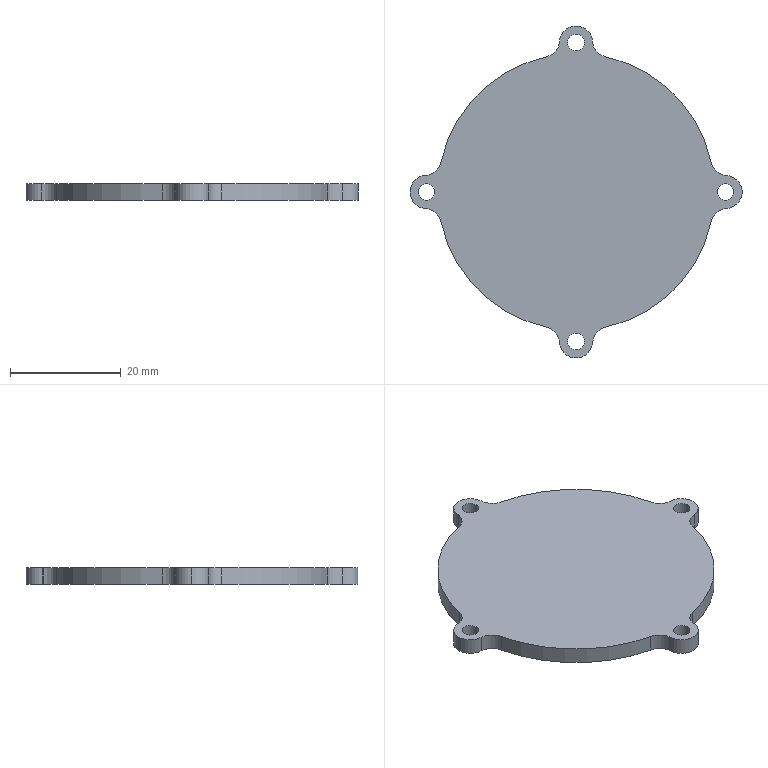Part | SolidWorks | features Extrusion 1 | 1 solid | 31 faces | box 60 x 60 x 3 mm | volume 6153 mm3 | cylinder 29 | plane 2 | commonest cylinder face diameters 6 x15 3 x8 50 x4 54 x2
STEP:
#1=CARTESIAN_POINT('',(-28.5,0.,3.));
#2=VERTEX_POINT('',#1);
#3=CARTESIAN_POINT('',(-25.5,0.,3.));
#4=VERTEX_POINT('',#3);
#5=CARTESIAN_POINT('',(-27.,0.,3.));
#6=DIRECTION('',(0.,0.,1.));
#7=DIRECTION('',(1.,0.,0.));
#8=AXIS2_PLACEMENT_3D('',#5,#6,#7);
#9=CIRCLE('',#8,1.5);
#10=EDGE_CURVE('',#2,#4,#9,.T.);
#11=ORIENTED_EDGE('',*,*,#10,.T.);
#12=CARTESIAN_POINT('',(-25.5,0.,0.));
#13=VERTEX_POINT('',#12);
#14=CARTESIAN_POINT('',(-25.5,0.,3.));
#15=DIRECTION('',(0.,0.,-1.));
#16=VECTOR('',#15,1000.);
#17=LINE('',#14,#16);
#18=EDGE_CURVE('',#4,#13,#17,.T.);
#19=ORIENTED_EDGE('',*,*,#18,.T.);
#20=CARTESIAN_POINT('',(-28.5,0.,0.));
#21=VERTEX_POINT('',#20);
#22=CARTESIAN_POINT('',(-27.,0.,0.));
#23=DIRECTION('',(0.,0.,1.));
#24=DIRECTION('',(1.,0.,0.));
#25=AXIS2_PLACEMENT_3D('',#22,#23,#24);
#26=CIRCLE('',#25,1.5);
#27=EDGE_CURVE('',#21,#13,#26,.T.);
#28=ORIENTED_EDGE('',*,*,#27,.F.);
#29=CARTESIAN_POINT('',(-28.5,0.,3.));
#30=DIRECTION('',(0.,0.,-1.));
#31=VECTOR('',#30,1000.);
#32=LINE('',#29,#31);
#33=EDGE_CURVE('',#2,#21,#32,.T.);
#34=ORIENTED_EDGE('',*,*,#33,.F.);
#35=EDGE_LOOP('',(#11,#19,#28,#34));
#36=FACE_OUTER_BOUND('',#35,.T.);
#37=CARTESIAN_POINT('',(-27.,0.,3.));
#38=DIRECTION('',(0.,0.,-1.));
#39=DIRECTION('',(-1.,0.,0.));
#40=AXIS2_PLACEMENT_3D('',#37,#38,#39);
#41=CYLINDRICAL_SURFACE('',#40,1.5);
#42=ADVANCED_FACE('',(#36),#41,.F.);
#43=CARTESIAN_POINT('',(-1.5,27.,3.));
#44=VERTEX_POINT('',#43);
#45=CARTESIAN_POINT('',(1.5,27.,3.));
#46=VERTEX_POINT('',#45);
#47=CARTESIAN_POINT('',(0.,27.,3.));
#48=DIRECTION('',(0.,0.,1.));
#49=DIRECTION('',(1.,0.,0.));
#50=AXIS2_PLACEMENT_3D('',#47,#48,#49);
#51=CIRCLE('',#50,1.5);
#52=EDGE_CURVE('',#44,#46,#51,.T.);
#53=ORIENTED_EDGE('',*,*,#52,.T.);
#54=CARTESIAN_POINT('',(1.5,27.,0.));
#55=VERTEX_POINT('',#54);
#56=CARTESIAN_POINT('',(1.5,27.,3.));
#57=DIRECTION('',(0.,0.,-1.));
#58=VECTOR('',#57,1000.);
#59=LINE('',#56,#58);
#60=EDGE_CURVE('',#46,#55,#59,.T.);
#61=ORIENTED_EDGE('',*,*,#60,.T.);
#62=CARTESIAN_POINT('',(-1.5,27.,0.));
#63=VERTEX_POINT('',#62);
#64=CARTESIAN_POINT('',(0.,27.,0.));
#65=DIRECTION('',(0.,0.,1.));
#66=DIRECTION('',(1.,0.,0.));
#67=AXIS2_PLACEMENT_3D('',#64,#65,#66);
#68=CIRCLE('',#67,1.5);
#69=EDGE_CURVE('',#63,#55,#68,.T.);
#70=ORIENTED_EDGE('',*,*,#69,.F.);
#71=CARTESIAN_POINT('',(-1.5,27.,3.));
#72=DIRECTION('',(0.,0.,-1.));
#73=VECTOR('',#72,1000.);
#74=LINE('',#71,#73);
#75=EDGE_CURVE('',#44,#63,#74,.T.);
#76=ORIENTED_EDGE('',*,*,#75,.F.);
#77=EDGE_LOOP('',(#53,#61,#70,#76));
#78=FACE_OUTER_BOUND('',#77,.T.);
#79=CARTESIAN_POINT('',(0.,27.,3.));
#80=DIRECTION('',(0.,0.,-1.));
#81=DIRECTION('',(-1.,0.,0.));
#82=AXIS2_PLACEMENT_3D('',#79,#80,#81);
#83=CYLINDRICAL_SURFACE('',#82,1.5);
#84=ADVANCED_FACE('',(#78),#83,.F.);
#85=CARTESIAN_POINT('',(25.5,0.,3.));
#86=VERTEX_POINT('',#85);
#87=CARTESIAN_POINT('',(28.5,0.,3.));
#88=VERTEX_POINT('',#87);
#89=CARTESIAN_POINT('',(27.,0.,3.));
#90=DIRECTION('',(0.,0.,1.));
#91=DIRECTION('',(1.,0.,0.));
#92=AXIS2_PLACEMENT_3D('',#89,#90,#91);
#93=CIRCLE('',#92,1.5);
#94=EDGE_CURVE('',#86,#88,#93,.T.);
#95=ORIENTED_EDGE('',*,*,#94,.T.);
#96=CARTESIAN_POINT('',(28.5,0.,0.));
#97=VERTEX_POINT('',#96);
#98=CARTESIAN_POINT('',(28.5,0.,3.));
#99=DIRECTION('',(0.,0.,-1.));
#100=VECTOR('',#99,1000.);
#101=LINE('',#98,#100);
#102=EDGE_CURVE('',#88,#97,#101,.T.);
#103=ORIENTED_EDGE('',*,*,#102,.T.);
#104=CARTESIAN_POINT('',(25.5,0.,0.));
#105=VERTEX_POINT('',#104);
#106=CARTESIAN_POINT('',(27.,0.,0.));
#107=DIRECTION('',(0.,0.,1.));
#108=DIRECTION('',(1.,0.,0.));
#109=AXIS2_PLACEMENT_3D('',#106,#107,#108);
#110=CIRCLE('',#109,1.5);
#111=EDGE_CURVE('',#105,#97,#110,.T.);
#112=ORIENTED_EDGE('',*,*,#111,.F.);
#113=CARTESIAN_POINT('',(25.5,0.,3.));
#114=DIRECTION('',(0.,0.,-1.));
#115=VECTOR('',#114,1000.);
#116=LINE('',#113,#115);
#117=EDGE_CURVE('',#86,#105,#116,.T.);
#118=ORIENTED_EDGE('',*,*,#117,.F.);
#119=EDGE_LOOP('',(#95,#103,#112,#118));
#120=FACE_OUTER_BOUND('',#119,.T.);
#121=CARTESIAN_POINT('',(27.,0.,3.));
#122=DIRECTION('',(0.,0.,-1.));
#123=DIRECTION('',(-1.,0.,0.));
#124=AXIS2_PLACEMENT_3D('',#121,#122,#123);
#125=CYLINDRICAL_SURFACE('',#124,1.5);
#126=ADVANCED_FACE('',(#120),#125,.F.);
#127=CARTESIAN_POINT('',(-1.5,-27.,3.));
#128=VERTEX_POINT('',#127);
#129=CARTESIAN_POINT('',(1.5,-27.,3.));
#130=VERTEX_POINT('',#129);
#131=CARTESIAN_POINT('',(0.,-27.,3.));
#132=DIRECTION('',(0.,0.,1.));
#133=DIRECTION('',(1.,0.,0.));
#134=AXIS2_PLACEMENT_3D('',#131,#132,#133);
#135=CIRCLE('',#134,1.5);
#136=EDGE_CURVE('',#128,#130,#135,.T.);
#137=ORIENTED_EDGE('',*,*,#136,.T.);
#138=CARTESIAN_POINT('',(1.5,-27.,0.));
#139=VERTEX_POINT('',#138);
#140=CARTESIAN_POINT('',(1.5,-27.,3.));
#141=DIRECTION('',(0.,0.,-1.));
#142=VECTOR('',#141,1000.);
#143=LINE('',#140,#142);
#144=EDGE_CURVE('',#130,#139,#143,.T.);
#145=ORIENTED_EDGE('',*,*,#144,.T.);
#146=CARTESIAN_POINT('',(-1.5,-27.,0.));
#147=VERTEX_POINT('',#146);
#148=CARTESIAN_POINT('',(0.,-27.,0.));
#149=DIRECTION('',(0.,0.,1.));
#150=DIRECTION('',(1.,0.,0.));
#151=AXIS2_PLACEMENT_3D('',#148,#149,#150);
#152=CIRCLE('',#151,1.5);
#153=EDGE_CURVE('',#147,#139,#152,.T.);
#154=ORIENTED_EDGE('',*,*,#153,.F.);
#155=CARTESIAN_POINT('',(-1.5,-27.,3.));
#156=DIRECTION('',(0.,0.,-1.));
#157=VECTOR('',#156,1000.);
#158=LINE('',#155,#157);
#159=EDGE_CURVE('',#128,#147,#158,.T.);
#160=ORIENTED_EDGE('',*,*,#159,.F.);
#161=EDGE_LOOP('',(#137,#145,#154,#160));
#162=FACE_OUTER_BOUND('',#161,.T.);
#163=CARTESIAN_POINT('',(0.,-27.,3.));
#164=DIRECTION('',(0.,0.,-1.));
#165=DIRECTION('',(-1.,0.,0.));
#166=AXIS2_PLACEMENT_3D('',#163,#164,#165);
#167=CYLINDRICAL_SURFACE('',#166,1.5);
#168=ADVANCED_FACE('',(#162),#167,.F.);
#169=CARTESIAN_POINT('',(-30.,0.,3.));
#170=VERTEX_POINT('',#169);
#171=CARTESIAN_POINT('',(-27.176,-2.995,3.));
#172=VERTEX_POINT('',#171);
#173=CARTESIAN_POINT('',(-27.,0.,3.));
#174=DIRECTION('',(0.,0.,1.));
#175=DIRECTION('',(1.,0.,0.));
#176=AXIS2_PLACEMENT_3D('',#173,#174,#175);
#177=CIRCLE('',#176,3.);
#178=EDGE_CURVE('',#170,#172,#177,.T.);
#179=ORIENTED_EDGE('',*,*,#178,.F.);
#180=CARTESIAN_POINT('',(-30.,0.,0.));
#181=VERTEX_POINT('',#180);
#182=CARTESIAN_POINT('',(-30.,0.,3.));
#183=DIRECTION('',(0.,0.,-1.));
#184=VECTOR('',#183,1000.);
#185=LINE('',#182,#184);
#186=EDGE_CURVE('',#170,#181,#185,.T.);
#187=ORIENTED_EDGE('',*,*,#186,.T.);
#188=CARTESIAN_POINT('',(-27.176,-2.995,0.));
#189=VERTEX_POINT('',#188);
#190=CARTESIAN_POINT('',(-27.,0.,0.));
#191=DIRECTION('',(0.,0.,1.));
#192=DIRECTION('',(1.,0.,0.));
#193=AXIS2_PLACEMENT_3D('',#190,#191,#192);
#194=CIRCLE('',#193,3.);
#195=EDGE_CURVE('',#181,#189,#194,.T.);
#196=ORIENTED_EDGE('',*,*,#195,.T.);
#197=CARTESIAN_POINT('',(-27.176,-2.995,3.));
#198=DIRECTION('',(0.,0.,-1.));
#199=VECTOR('',#198,1000.);
#200=LINE('',#197,#199);
#201=EDGE_CURVE('',#172,#189,#200,.T.);
#202=ORIENTED_EDGE('',*,*,#201,.F.);
#203=EDGE_LOOP('',(#179,#187,#196,#202));
#204=FACE_OUTER_BOUND('',#203,.T.);
#205=CARTESIAN_POINT('',(-27.,0.,3.));
#206=DIRECTION('',(0.,0.,-1.));
#207=DIRECTION('',(-1.,0.,0.));
#208=AXIS2_PLACEMENT_3D('',#205,#206,#207);
#209=CYLINDRICAL_SURFACE('',#208,3.);
#210=ADVANCED_FACE('',(#204),#209,.T.);
#211=CARTESIAN_POINT('',(3.,27.,3.));
#212=VERTEX_POINT('',#211);
#213=CARTESIAN_POINT('',(-3.,27.,3.));
#214=VERTEX_POINT('',#213);
#215=CARTESIAN_POINT('',(0.,27.,3.));
#216=DIRECTION('',(0.,0.,1.));
#217=DIRECTION('',(1.,0.,0.));
#218=AXIS2_PLACEMENT_3D('',#215,#216,#217);
#219=CIRCLE('',#218,3.);
#220=EDGE_CURVE('',#212,#214,#219,.T.);
#221=ORIENTED_EDGE('',*,*,#220,.F.);
#222=CARTESIAN_POINT('',(3.,27.,0.));
#223=VERTEX_POINT('',#222);
#224=CARTESIAN_POINT('',(3.,27.,3.));
#225=DIRECTION('',(0.,0.,-1.));
#226=VECTOR('',#225,1000.);
#227=LINE('',#224,#226);
#228=EDGE_CURVE('',#212,#223,#227,.T.);
#229=ORIENTED_EDGE('',*,*,#228,.T.);
#230=CARTESIAN_POINT('',(-3.,27.,0.));
#231=VERTEX_POINT('',#230);
#232=CARTESIAN_POINT('',(0.,27.,0.));
#233=DIRECTION('',(0.,0.,1.));
#234=DIRECTION('',(1.,0.,0.));
#235=AXIS2_PLACEMENT_3D('',#232,#233,#234);
#236=CIRCLE('',#235,3.);
#237=EDGE_CURVE('',#223,#231,#236,.T.);
#238=ORIENTED_EDGE('',*,*,#237,.T.);
#239=CARTESIAN_POINT('',(-3.,27.,3.));
#240=DIRECTION('',(0.,0.,-1.));
#241=VECTOR('',#240,1000.);
#242=LINE('',#239,#241);
#243=EDGE_CURVE('',#214,#231,#242,.T.);
#244=ORIENTED_EDGE('',*,*,#243,.F.);
#245=EDGE_LOOP('',(#221,#229,#238,#244));
#246=FACE_OUTER_BOUND('',#245,.T.);
#247=CARTESIAN_POINT('',(0.,27.,3.));
#248=DIRECTION('',(0.,0.,-1.));
#249=DIRECTION('',(-1.,0.,0.));
#250=AXIS2_PLACEMENT_3D('',#247,#248,#249);
#251=CYLINDRICAL_SURFACE('',#250,3.);
#252=ADVANCED_FACE('',(#246),#251,.T.);
#253=CARTESIAN_POINT('',(-2.995,26.833,3.));
#254=VERTEX_POINT('',#253);
#255=CARTESIAN_POINT('',(0.,27.,3.));
#256=DIRECTION('',(0.,0.,1.));
#257=DIRECTION('',(1.,0.,0.));
#258=AXIS2_PLACEMENT_3D('',#255,#256,#257);
#259=CIRCLE('',#258,3.);
#260=EDGE_CURVE('',#214,#254,#259,.T.);
#261=ORIENTED_EDGE('',*,*,#260,.F.);
#262=ORIENTED_EDGE('',*,*,#243,.T.);
#263=CARTESIAN_POINT('',(-2.995,26.833,0.));
#264=VERTEX_POINT('',#263);
#265=CARTESIAN_POINT('',(0.,27.,0.));
#266=DIRECTION('',(0.,0.,1.));
#267=DIRECTION('',(1.,0.,0.));
#268=AXIS2_PLACEMENT_3D('',#265,#266,#267);
#269=CIRCLE('',#268,3.);
#270=EDGE_CURVE('',#231,#264,#269,.T.);
#271=ORIENTED_EDGE('',*,*,#270,.T.);
#272=CARTESIAN_POINT('',(-2.995,26.833,3.));
#273=DIRECTION('',(0.,0.,-1.));
#274=VECTOR('',#273,1000.);
#275=LINE('',#272,#274);
#276=EDGE_CURVE('',#254,#264,#275,.T.);
#277=ORIENTED_EDGE('',*,*,#276,.F.);
#278=EDGE_LOOP('',(#261,#262,#271,#277));
#279=FACE_OUTER_BOUND('',#278,.T.);
#280=CARTESIAN_POINT('',(0.,27.,3.));
#281=DIRECTION('',(0.,0.,-1.));
#282=DIRECTION('',(-1.,0.,0.));
#283=AXIS2_PLACEMENT_3D('',#280,#281,#282);
#284=CYLINDRICAL_SURFACE('',#283,3.);
#285=ADVANCED_FACE('',(#279),#284,.T.);
#286=CARTESIAN_POINT('',(24.421,-5.348,0.));
#287=VERTEX_POINT('',#286);
#288=CARTESIAN_POINT('',(27.176,-2.995,0.));
#289=VERTEX_POINT('',#288);
#290=CARTESIAN_POINT('',(27.352,-5.99,0.));
#291=DIRECTION('',(0.,0.,-1.));
#292=DIRECTION('',(1.,0.,0.));
#293=AXIS2_PLACEMENT_3D('',#290,#291,#292);
#294=CIRCLE('',#293,3.);
#295=EDGE_CURVE('',#287,#289,#294,.T.);
#296=ORIENTED_EDGE('',*,*,#295,.T.);
#297=CARTESIAN_POINT('',(27.176,-2.995,3.));
#298=VERTEX_POINT('',#297);
#299=CARTESIAN_POINT('',(27.176,-2.995,3.));
#300=DIRECTION('',(0.,0.,-1.));
#301=VECTOR('',#300,1000.);
#302=LINE('',#299,#301);
#303=EDGE_CURVE('',#298,#289,#302,.T.);
#304=ORIENTED_EDGE('',*,*,#303,.F.);
#305=CARTESIAN_POINT('',(24.421,-5.348,3.));
#306=VERTEX_POINT('',#305);
#307=CARTESIAN_POINT('',(27.352,-5.99,3.));
#308=DIRECTION('',(0.,0.,-1.));
#309=DIRECTION('',(1.,0.,0.));
#310=AXIS2_PLACEMENT_3D('',#307,#308,#309);
#311=CIRCLE('',#310,3.);
#312=EDGE_CURVE('',#306,#298,#311,.T.);
#313=ORIENTED_EDGE('',*,*,#312,.F.);
#314=CARTESIAN_POINT('',(24.421,-5.348,3.));
#315=DIRECTION('',(0.,0.,-1.));
#316=VECTOR('',#315,1000.);
#317=LINE('',#314,#316);
#318=EDGE_CURVE('',#306,#287,#317,.T.);
#319=ORIENTED_EDGE('',*,*,#318,.T.);
#320=EDGE_LOOP('',(#296,#304,#313,#319));
#321=FACE_OUTER_BOUND('',#320,.T.);
#322=CARTESIAN_POINT('',(27.352,-5.99,3.));
#323=DIRECTION('',(0.,0.,-1.));
#324=DIRECTION('',(-1.,0.,0.));
#325=AXIS2_PLACEMENT_3D('',#322,#323,#324);
#326=CYLINDRICAL_SURFACE('',#325,3.);
#327=ADVANCED_FACE('',(#321),#326,.F.);
#328=CARTESIAN_POINT('',(27.176,2.995,0.));
#329=VERTEX_POINT('',#328);
#330=CARTESIAN_POINT('',(27.,0.,0.));
#331=DIRECTION('',(0.,0.,1.));
#332=DIRECTION('',(1.,0.,0.));
#333=AXIS2_PLACEMENT_3D('',#330,#331,#332);
#334=CIRCLE('',#333,3.);
#335=EDGE_CURVE('',#289,#329,#334,.T.);
#336=ORIENTED_EDGE('',*,*,#335,.T.);
#337=CARTESIAN_POINT('',(27.176,2.995,3.));
#338=VERTEX_POINT('',#337);
#339=CARTESIAN_POINT('',(27.176,2.995,3.));
#340=DIRECTION('',(0.,0.,-1.));
#341=VECTOR('',#340,1000.);
#342=LINE('',#339,#341);
#343=EDGE_CURVE('',#338,#329,#342,.T.);
#344=ORIENTED_EDGE('',*,*,#343,.F.);
#345=CARTESIAN_POINT('',(27.,0.,3.));
#346=DIRECTION('',(0.,0.,1.));
#347=DIRECTION('',(1.,0.,0.));
#348=AXIS2_PLACEMENT_3D('',#345,#346,#347);
#349=CIRCLE('',#348,3.);
#350=EDGE_CURVE('',#298,#338,#349,.T.);
#351=ORIENTED_EDGE('',*,*,#350,.F.);
#352=ORIENTED_EDGE('',*,*,#303,.T.);
#353=EDGE_LOOP('',(#336,#344,#351,#352));
#354=FACE_OUTER_BOUND('',#353,.T.);
#355=CARTESIAN_POINT('',(27.,0.,3.));
#356=DIRECTION('',(0.,0.,-1.));
#357=DIRECTION('',(-1.,0.,0.));
#358=AXIS2_PLACEMENT_3D('',#355,#356,#357);
#359=CYLINDRICAL_SURFACE('',#358,3.);
#360=ADVANCED_FACE('',(#354),#359,.T.);
#361=CARTESIAN_POINT('',(24.421,5.348,0.));
#362=VERTEX_POINT('',#361);
#363=CARTESIAN_POINT('',(27.352,5.99,0.));
#364=DIRECTION('',(0.,0.,1.));
#365=DIRECTION('',(1.,0.,0.));
#366=AXIS2_PLACEMENT_3D('',#363,#364,#365);
#367=CIRCLE('',#366,3.);
#368=EDGE_CURVE('',#362,#329,#367,.T.);
#369=ORIENTED_EDGE('',*,*,#368,.F.);
#370=CARTESIAN_POINT('',(24.421,5.348,3.));
#371=VERTEX_POINT('',#370);
#372=CARTESIAN_POINT('',(24.421,5.348,3.));
#373=DIRECTION('',(0.,0.,-1.));
#374=VECTOR('',#373,1000.);
#375=LINE('',#372,#374);
#376=EDGE_CURVE('',#371,#362,#375,.T.);
#377=ORIENTED_EDGE('',*,*,#376,.F.);
#378=CARTESIAN_POINT('',(27.352,5.99,3.));
#379=DIRECTION('',(0.,0.,1.));
#380=DIRECTION('',(1.,0.,0.));
#381=AXIS2_PLACEMENT_3D('',#378,#379,#380);
#382=CIRCLE('',#381,3.);
#383=EDGE_CURVE('',#371,#338,#382,.T.);
#384=ORIENTED_EDGE('',*,*,#383,.T.);
#385=ORIENTED_EDGE('',*,*,#343,.T.);
#386=EDGE_LOOP('',(#369,#377,#384,#385));
#387=FACE_OUTER_BOUND('',#386,.T.);
#388=CARTESIAN_POINT('',(27.352,5.99,3.));
#389=DIRECTION('',(0.,0.,-1.));
#390=DIRECTION('',(-1.,0.,0.));
#391=AXIS2_PLACEMENT_3D('',#388,#389,#390);
#392=CYLINDRICAL_SURFACE('',#391,3.);
#393=ADVANCED_FACE('',(#387),#392,.F.);
#394=CARTESIAN_POINT('',(5.348,24.421,0.));
#395=VERTEX_POINT('',#394);
#396=CARTESIAN_POINT('',(0.,0.,0.));
#397=DIRECTION('',(0.,0.,1.));
#398=DIRECTION('',(1.,0.,0.));
#399=AXIS2_PLACEMENT_3D('',#396,#397,#398);
#400=CIRCLE('',#399,25.);
#401=EDGE_CURVE('',#362,#395,#400,.T.);
#402=ORIENTED_EDGE('',*,*,#401,.T.);
#403=CARTESIAN_POINT('',(5.348,24.421,3.));
#404=VERTEX_POINT('',#403);
#405=CARTESIAN_POINT('',(5.348,24.421,3.));
#406=DIRECTION('',(0.,0.,-1.));
#407=VECTOR('',#406,1000.);
#408=LINE('',#405,#407);
#409=EDGE_CURVE('',#404,#395,#408,.T.);
#410=ORIENTED_EDGE('',*,*,#409,.F.);
#411=CARTESIAN_POINT('',(0.,0.,3.));
#412=DIRECTION('',(0.,0.,1.));
#413=DIRECTION('',(1.,0.,0.));
#414=AXIS2_PLACEMENT_3D('',#411,#412,#413);
#415=CIRCLE('',#414,25.);
#416=EDGE_CURVE('',#371,#404,#415,.T.);
#417=ORIENTED_EDGE('',*,*,#416,.F.);
#418=ORIENTED_EDGE('',*,*,#376,.T.);
#419=EDGE_LOOP('',(#402,#410,#417,#418));
#420=FACE_OUTER_BOUND('',#419,.T.);
#421=CARTESIAN_POINT('',(0.,0.,3.));
#422=DIRECTION('',(0.,0.,-1.));
#423=DIRECTION('',(-1.,0.,0.));
#424=AXIS2_PLACEMENT_3D('',#421,#422,#423);
#425=CYLINDRICAL_SURFACE('',#424,25.);
#426=ADVANCED_FACE('',(#420),#425,.T.);
#427=CARTESIAN_POINT('',(3.036,26.829,0.));
#428=VERTEX_POINT('',#427);
#429=CARTESIAN_POINT('',(5.99,27.352,0.));
#430=DIRECTION('',(0.,0.,-1.));
#431=DIRECTION('',(1.,0.,0.));
#432=AXIS2_PLACEMENT_3D('',#429,#430,#431);
#433=CIRCLE('',#432,3.);
#434=EDGE_CURVE('',#395,#428,#433,.T.);
#435=ORIENTED_EDGE('',*,*,#434,.T.);
#436=CARTESIAN_POINT('',(3.036,26.829,3.));
#437=VERTEX_POINT('',#436);
#438=CARTESIAN_POINT('',(3.036,26.829,3.));
#439=DIRECTION('',(0.,0.,-1.));
#440=VECTOR('',#439,1000.);
#441=LINE('',#438,#440);
#442=EDGE_CURVE('',#437,#428,#441,.T.);
#443=ORIENTED_EDGE('',*,*,#442,.F.);
#444=CARTESIAN_POINT('',(5.99,27.352,3.));
#445=DIRECTION('',(0.,0.,-1.));
#446=DIRECTION('',(1.,0.,0.));
#447=AXIS2_PLACEMENT_3D('',#444,#445,#446);
#448=CIRCLE('',#447,3.);
#449=EDGE_CURVE('',#404,#437,#448,.T.);
#450=ORIENTED_EDGE('',*,*,#449,.F.);
#451=ORIENTED_EDGE('',*,*,#409,.T.);
#452=EDGE_LOOP('',(#435,#443,#450,#451));
#453=FACE_OUTER_BOUND('',#452,.T.);
#454=CARTESIAN_POINT('',(5.99,27.352,3.));
#455=DIRECTION('',(0.,0.,-1.));
#456=DIRECTION('',(-1.,0.,0.));
#457=AXIS2_PLACEMENT_3D('',#454,#455,#456);
#458=CYLINDRICAL_SURFACE('',#457,3.);
#459=ADVANCED_FACE('',(#453),#458,.F.);
#460=CARTESIAN_POINT('',(2.995,26.833,0.));
#461=VERTEX_POINT('',#460);
#462=CARTESIAN_POINT('',(0.,0.,0.));
#463=DIRECTION('',(0.,0.,1.));
#464=DIRECTION('',(1.,0.,0.));
#465=AXIS2_PLACEMENT_3D('',#462,#463,#464);
#466=CIRCLE('',#465,27.);
#467=EDGE_CURVE('',#428,#461,#466,.T.);
#468=ORIENTED_EDGE('',*,*,#467,.T.);
#469=CARTESIAN_POINT('',(2.995,26.833,3.));
#470=VERTEX_POINT('',#469);
#471=CARTESIAN_POINT('',(2.995,26.833,3.));
#472=DIRECTION('',(0.,0.,-1.));
#473=VECTOR('',#472,1000.);
#474=LINE('',#471,#473);
#475=EDGE_CURVE('',#470,#461,#474,.T.);
#476=ORIENTED_EDGE('',*,*,#475,.F.);
#477=CARTESIAN_POINT('',(0.,0.,3.));
#478=DIRECTION('',(0.,0.,1.));
#479=DIRECTION('',(1.,0.,0.));
#480=AXIS2_PLACEMENT_3D('',#477,#478,#479);
#481=CIRCLE('',#480,27.);
#482=EDGE_CURVE('',#437,#470,#481,.T.);
#483=ORIENTED_EDGE('',*,*,#482,.F.);
#484=ORIENTED_EDGE('',*,*,#442,.T.);
#485=EDGE_LOOP('',(#468,#476,#483,#484));
#486=FACE_OUTER_BOUND('',#485,.T.);
#487=CARTESIAN_POINT('',(0.,0.,3.));
#488=DIRECTION('',(0.,0.,-1.));
#489=DIRECTION('',(-1.,0.,0.));
#490=AXIS2_PLACEMENT_3D('',#487,#488,#489);
#491=CYLINDRICAL_SURFACE('',#490,27.);
#492=ADVANCED_FACE('',(#486),#491,.T.);
#493=ORIENTED_EDGE('',*,*,#228,.F.);
#494=CARTESIAN_POINT('',(0.,27.,3.));
#495=DIRECTION('',(0.,0.,1.));
#496=DIRECTION('',(1.,0.,0.));
#497=AXIS2_PLACEMENT_3D('',#494,#495,#496);
#498=CIRCLE('',#497,3.);
#499=EDGE_CURVE('',#470,#212,#498,.T.);
#500=ORIENTED_EDGE('',*,*,#499,.F.);
#501=ORIENTED_EDGE('',*,*,#475,.T.);
#502=CARTESIAN_POINT('',(0.,27.,0.));
#503=DIRECTION('',(0.,0.,1.));
#504=DIRECTION('',(1.,0.,0.));
#505=AXIS2_PLACEMENT_3D('',#502,#503,#504);
#506=CIRCLE('',#505,3.);
#507=EDGE_CURVE('',#461,#223,#506,.T.);
#508=ORIENTED_EDGE('',*,*,#507,.T.);
#509=EDGE_LOOP('',(#493,#500,#501,#508));
#510=FACE_OUTER_BOUND('',#509,.T.);
#511=CARTESIAN_POINT('',(0.,27.,3.));
#512=DIRECTION('',(0.,0.,-1.));
#513=DIRECTION('',(-1.,0.,0.));
#514=AXIS2_PLACEMENT_3D('',#511,#512,#513);
#515=CYLINDRICAL_SURFACE('',#514,3.);
#516=ADVANCED_FACE('',(#510),#515,.T.);
#517=CARTESIAN_POINT('',(-3.036,26.829,0.));
#518=VERTEX_POINT('',#517);
#519=CARTESIAN_POINT('',(0.,0.,0.));
#520=DIRECTION('',(0.,0.,1.));
#521=DIRECTION('',(1.,0.,0.));
#522=AXIS2_PLACEMENT_3D('',#519,#520,#521);
#523=CIRCLE('',#522,27.);
#524=EDGE_CURVE('',#264,#518,#523,.T.);
#525=ORIENTED_EDGE('',*,*,#524,.T.);
#526=CARTESIAN_POINT('',(-3.036,26.829,3.));
#527=VERTEX_POINT('',#526);
#528=CARTESIAN_POINT('',(-3.036,26.829,3.));
#529=DIRECTION('',(0.,0.,-1.));
#530=VECTOR('',#529,1000.);
#531=LINE('',#528,#530);
#532=EDGE_CURVE('',#527,#518,#531,.T.);
#533=ORIENTED_EDGE('',*,*,#532,.F.);
#534=CARTESIAN_POINT('',(0.,0.,3.));
#535=DIRECTION('',(0.,0.,1.));
#536=DIRECTION('',(1.,0.,0.));
#537=AXIS2_PLACEMENT_3D('',#534,#535,#536);
#538=CIRCLE('',#537,27.);
#539=EDGE_CURVE('',#254,#527,#538,.T.);
#540=ORIENTED_EDGE('',*,*,#539,.F.);
#541=ORIENTED_EDGE('',*,*,#276,.T.);
#542=EDGE_LOOP('',(#525,#533,#540,#541));
#543=FACE_OUTER_BOUND('',#542,.T.);
#544=CARTESIAN_POINT('',(0.,0.,3.));
#545=DIRECTION('',(0.,0.,-1.));
#546=DIRECTION('',(-1.,0.,0.));
#547=AXIS2_PLACEMENT_3D('',#544,#545,#546);
#548=CYLINDRICAL_SURFACE('',#547,27.);
#549=ADVANCED_FACE('',(#543),#548,.T.);
#550=CARTESIAN_POINT('',(-5.348,24.421,0.));
#551=VERTEX_POINT('',#550);
#552=CARTESIAN_POINT('',(-5.99,27.352,0.));
#553=DIRECTION('',(0.,0.,1.));
#554=DIRECTION('',(1.,0.,0.));
#555=AXIS2_PLACEMENT_3D('',#552,#553,#554);
#556=CIRCLE('',#555,3.);
#557=EDGE_CURVE('',#551,#518,#556,.T.);
#558=ORIENTED_EDGE('',*,*,#557,.F.);
#559=CARTESIAN_POINT('',(-5.348,24.421,3.));
#560=VERTEX_POINT('',#559);
#561=CARTESIAN_POINT('',(-5.348,24.421,3.));
#562=DIRECTION('',(0.,0.,-1.));
#563=VECTOR('',#562,1000.);
#564=LINE('',#561,#563);
#565=EDGE_CURVE('',#560,#551,#564,.T.);
#566=ORIENTED_EDGE('',*,*,#565,.F.);
#567=CARTESIAN_POINT('',(-5.99,27.352,3.));
#568=DIRECTION('',(0.,0.,1.));
#569=DIRECTION('',(1.,0.,0.));
#570=AXIS2_PLACEMENT_3D('',#567,#568,#569);
#571=CIRCLE('',#570,3.);
#572=EDGE_CURVE('',#560,#527,#571,.T.);
#573=ORIENTED_EDGE('',*,*,#572,.T.);
#574=ORIENTED_EDGE('',*,*,#532,.T.);
#575=EDGE_LOOP('',(#558,#566,#573,#574));
#576=FACE_OUTER_BOUND('',#575,.T.);
#577=CARTESIAN_POINT('',(-5.99,27.352,3.));
#578=DIRECTION('',(0.,0.,-1.));
#579=DIRECTION('',(-1.,0.,0.));
#580=AXIS2_PLACEMENT_3D('',#577,#578,#579);
#581=CYLINDRICAL_SURFACE('',#580,3.);
#582=ADVANCED_FACE('',(#576),#581,.F.);
#583=CARTESIAN_POINT('',(-24.421,5.348,0.));
#584=VERTEX_POINT('',#583);
#585=CARTESIAN_POINT('',(0.,0.,0.));
#586=DIRECTION('',(0.,0.,1.));
#587=DIRECTION('',(1.,0.,0.));
#588=AXIS2_PLACEMENT_3D('',#585,#586,#587);
#589=CIRCLE('',#588,25.);
#590=EDGE_CURVE('',#551,#584,#589,.T.);
#591=ORIENTED_EDGE('',*,*,#590,.T.);
#592=CARTESIAN_POINT('',(-24.421,5.348,3.));
#593=VERTEX_POINT('',#592);
#594=CARTESIAN_POINT('',(-24.421,5.348,3.));
#595=DIRECTION('',(0.,0.,-1.));
#596=VECTOR('',#595,1000.);
#597=LINE('',#594,#596);
#598=EDGE_CURVE('',#593,#584,#597,.T.);
#599=ORIENTED_EDGE('',*,*,#598,.F.);
#600=CARTESIAN_POINT('',(0.,0.,3.));
#601=DIRECTION('',(0.,0.,1.));
#602=DIRECTION('',(1.,0.,0.));
#603=AXIS2_PLACEMENT_3D('',#600,#601,#602);
#604=CIRCLE('',#603,25.);
#605=EDGE_CURVE('',#560,#593,#604,.T.);
#606=ORIENTED_EDGE('',*,*,#605,.F.);
#607=ORIENTED_EDGE('',*,*,#565,.T.);
#608=EDGE_LOOP('',(#591,#599,#606,#607));
#609=FACE_OUTER_BOUND('',#608,.T.);
#610=CARTESIAN_POINT('',(0.,0.,3.));
#611=DIRECTION('',(0.,0.,-1.));
#612=DIRECTION('',(-1.,0.,0.));
#613=AXIS2_PLACEMENT_3D('',#610,#611,#612);
#614=CYLINDRICAL_SURFACE('',#613,25.);
#615=ADVANCED_FACE('',(#609),#614,.T.);
#616=CARTESIAN_POINT('',(-27.176,2.995,0.));
#617=VERTEX_POINT('',#616);
#618=CARTESIAN_POINT('',(-27.352,5.99,0.));
#619=DIRECTION('',(0.,0.,-1.));
#620=DIRECTION('',(1.,0.,0.));
#621=AXIS2_PLACEMENT_3D('',#618,#619,#620);
#622=CIRCLE('',#621,3.);
#623=EDGE_CURVE('',#584,#617,#622,.T.);
#624=ORIENTED_EDGE('',*,*,#623,.T.);
#625=CARTESIAN_POINT('',(-27.176,2.995,3.));
#626=VERTEX_POINT('',#625);
#627=CARTESIAN_POINT('',(-27.176,2.995,3.));
#628=DIRECTION('',(0.,0.,-1.));
#629=VECTOR('',#628,1000.);
#630=LINE('',#627,#629);
#631=EDGE_CURVE('',#626,#617,#630,.T.);
#632=ORIENTED_EDGE('',*,*,#631,.F.);
#633=CARTESIAN_POINT('',(-27.352,5.99,3.));
#634=DIRECTION('',(0.,0.,-1.));
#635=DIRECTION('',(1.,0.,0.));
#636=AXIS2_PLACEMENT_3D('',#633,#634,#635);
#637=CIRCLE('',#636,3.);
#638=EDGE_CURVE('',#593,#626,#637,.T.);
#639=ORIENTED_EDGE('',*,*,#638,.F.);
#640=ORIENTED_EDGE('',*,*,#598,.T.);
#641=EDGE_LOOP('',(#624,#632,#639,#640));
#642=FACE_OUTER_BOUND('',#641,.T.);
#643=CARTESIAN_POINT('',(-27.352,5.99,3.));
#644=DIRECTION('',(0.,0.,-1.));
#645=DIRECTION('',(-1.,0.,0.));
#646=AXIS2_PLACEMENT_3D('',#643,#644,#645);
#647=CYLINDRICAL_SURFACE('',#646,3.);
#648=ADVANCED_FACE('',(#642),#647,.F.);
#649=ORIENTED_EDGE('',*,*,#186,.F.);
#650=CARTESIAN_POINT('',(-27.,0.,3.));
#651=DIRECTION('',(0.,0.,1.));
#652=DIRECTION('',(1.,0.,0.));
#653=AXIS2_PLACEMENT_3D('',#650,#651,#652);
#654=CIRCLE('',#653,3.);
#655=EDGE_CURVE('',#626,#170,#654,.T.);
#656=ORIENTED_EDGE('',*,*,#655,.F.);
#657=ORIENTED_EDGE('',*,*,#631,.T.);
#658=CARTESIAN_POINT('',(-27.,0.,0.));
#659=DIRECTION('',(0.,0.,1.));
#660=DIRECTION('',(1.,0.,0.));
#661=AXIS2_PLACEMENT_3D('',#658,#659,#660);
#662=CIRCLE('',#661,3.);
#663=EDGE_CURVE('',#617,#181,#662,.T.);
#664=ORIENTED_EDGE('',*,*,#663,.T.);
#665=EDGE_LOOP('',(#649,#656,#657,#664));
#666=FACE_OUTER_BOUND('',#665,.T.);
#667=CARTESIAN_POINT('',(-27.,0.,3.));
#668=DIRECTION('',(0.,0.,-1.));
#669=DIRECTION('',(-1.,0.,0.));
#670=AXIS2_PLACEMENT_3D('',#667,#668,#669);
#671=CYLINDRICAL_SURFACE('',#670,3.);
#672=ADVANCED_FACE('',(#666),#671,.T.);
#673=CARTESIAN_POINT('',(-24.421,-5.348,0.));
#674=VERTEX_POINT('',#673);
#675=CARTESIAN_POINT('',(-27.352,-5.99,0.));
#676=DIRECTION('',(0.,0.,1.));
#677=DIRECTION('',(1.,0.,0.));
#678=AXIS2_PLACEMENT_3D('',#675,#676,#677);
#679=CIRCLE('',#678,3.);
#680=EDGE_CURVE('',#674,#189,#679,.T.);
#681=ORIENTED_EDGE('',*,*,#680,.F.);
#682=CARTESIAN_POINT('',(-24.421,-5.348,3.));
#683=VERTEX_POINT('',#682);
#684=CARTESIAN_POINT('',(-24.421,-5.348,3.));
#685=DIRECTION('',(0.,0.,-1.));
#686=VECTOR('',#685,1000.);
#687=LINE('',#684,#686);
#688=EDGE_CURVE('',#683,#674,#687,.T.);
#689=ORIENTED_EDGE('',*,*,#688,.F.);
#690=CARTESIAN_POINT('',(-27.352,-5.99,3.));
#691=DIRECTION('',(0.,0.,1.));
#692=DIRECTION('',(1.,0.,0.));
#693=AXIS2_PLACEMENT_3D('',#690,#691,#692);
#694=CIRCLE('',#693,3.);
#695=EDGE_CURVE('',#683,#172,#694,.T.);
#696=ORIENTED_EDGE('',*,*,#695,.T.);
#697=ORIENTED_EDGE('',*,*,#201,.T.);
#698=EDGE_LOOP('',(#681,#689,#696,#697));
#699=FACE_OUTER_BOUND('',#698,.T.);
#700=CARTESIAN_POINT('',(-27.352,-5.99,3.));
#701=DIRECTION('',(0.,0.,-1.));
#702=DIRECTION('',(-1.,0.,0.));
#703=AXIS2_PLACEMENT_3D('',#700,#701,#702);
#704=CYLINDRICAL_SURFACE('',#703,3.);
#705=ADVANCED_FACE('',(#699),#704,.F.);
#706=CARTESIAN_POINT('',(-5.348,-24.421,0.));
#707=VERTEX_POINT('',#706);
#708=CARTESIAN_POINT('',(0.,0.,0.));
#709=DIRECTION('',(0.,0.,1.));
#710=DIRECTION('',(1.,0.,0.));
#711=AXIS2_PLACEMENT_3D('',#708,#709,#710);
#712=CIRCLE('',#711,25.);
#713=EDGE_CURVE('',#674,#707,#712,.T.);
#714=ORIENTED_EDGE('',*,*,#713,.T.);
#715=CARTESIAN_POINT('',(-5.348,-24.421,3.));
#716=VERTEX_POINT('',#715);
#717=CARTESIAN_POINT('',(-5.348,-24.421,3.));
#718=DIRECTION('',(0.,0.,-1.));
#719=VECTOR('',#718,1000.);
#720=LINE('',#717,#719);
#721=EDGE_CURVE('',#716,#707,#720,.T.);
#722=ORIENTED_EDGE('',*,*,#721,.F.);
#723=CARTESIAN_POINT('',(0.,0.,3.));
#724=DIRECTION('',(0.,0.,1.));
#725=DIRECTION('',(1.,0.,0.));
#726=AXIS2_PLACEMENT_3D('',#723,#724,#725);
#727=CIRCLE('',#726,25.);
#728=EDGE_CURVE('',#683,#716,#727,.T.);
#729=ORIENTED_EDGE('',*,*,#728,.F.);
#730=ORIENTED_EDGE('',*,*,#688,.T.);
#731=EDGE_LOOP('',(#714,#722,#729,#730));
#732=FACE_OUTER_BOUND('',#731,.T.);
#733=CARTESIAN_POINT('',(0.,0.,3.));
#734=DIRECTION('',(0.,0.,-1.));
#735=DIRECTION('',(-1.,0.,0.));
#736=AXIS2_PLACEMENT_3D('',#733,#734,#735);
#737=CYLINDRICAL_SURFACE('',#736,25.);
#738=ADVANCED_FACE('',(#732),#737,.T.);
#739=CARTESIAN_POINT('',(-2.995,-27.176,0.));
#740=VERTEX_POINT('',#739);
#741=CARTESIAN_POINT('',(-5.99,-27.352,0.));
#742=DIRECTION('',(0.,0.,-1.));
#743=DIRECTION('',(1.,0.,0.));
#744=AXIS2_PLACEMENT_3D('',#741,#742,#743);
#745=CIRCLE('',#744,3.);
#746=EDGE_CURVE('',#707,#740,#745,.T.);
#747=ORIENTED_EDGE('',*,*,#746,.T.);
#748=CARTESIAN_POINT('',(-2.995,-27.176,3.));
#749=VERTEX_POINT('',#748);
#750=CARTESIAN_POINT('',(-2.995,-27.176,3.));
#751=DIRECTION('',(0.,0.,-1.));
#752=VECTOR('',#751,1000.);
#753=LINE('',#750,#752);
#754=EDGE_CURVE('',#749,#740,#753,.T.);
#755=ORIENTED_EDGE('',*,*,#754,.F.);
#756=CARTESIAN_POINT('',(-5.99,-27.352,3.));
#757=DIRECTION('',(0.,0.,-1.));
#758=DIRECTION('',(1.,0.,0.));
#759=AXIS2_PLACEMENT_3D('',#756,#757,#758);
#760=CIRCLE('',#759,3.);
#761=EDGE_CURVE('',#716,#749,#760,.T.);
#762=ORIENTED_EDGE('',*,*,#761,.F.);
#763=ORIENTED_EDGE('',*,*,#721,.T.);
#764=EDGE_LOOP('',(#747,#755,#762,#763));
#765=FACE_OUTER_BOUND('',#764,.T.);
#766=CARTESIAN_POINT('',(-5.99,-27.352,3.));
#767=DIRECTION('',(0.,0.,-1.));
#768=DIRECTION('',(-1.,0.,0.));
#769=AXIS2_PLACEMENT_3D('',#766,#767,#768);
#770=CYLINDRICAL_SURFACE('',#769,3.);
#771=ADVANCED_FACE('',(#765),#770,.F.);
#772=CARTESIAN_POINT('',(2.995,-27.176,0.));
#773=VERTEX_POINT('',#772);
#774=CARTESIAN_POINT('',(0.,-27.,0.));
#775=DIRECTION('',(0.,0.,1.));
#776=DIRECTION('',(1.,0.,0.));
#777=AXIS2_PLACEMENT_3D('',#774,#775,#776);
#778=CIRCLE('',#777,3.);
#779=EDGE_CURVE('',#740,#773,#778,.T.);
#780=ORIENTED_EDGE('',*,*,#779,.T.);
#781=CARTESIAN_POINT('',(2.995,-27.176,3.));
#782=VERTEX_POINT('',#781);
#783=CARTESIAN_POINT('',(2.995,-27.176,3.));
#784=DIRECTION('',(0.,0.,-1.));
#785=VECTOR('',#784,1000.);
#786=LINE('',#783,#785);
#787=EDGE_CURVE('',#782,#773,#786,.T.);
#788=ORIENTED_EDGE('',*,*,#787,.F.);
#789=CARTESIAN_POINT('',(0.,-27.,3.));
#790=DIRECTION('',(0.,0.,1.));
#791=DIRECTION('',(1.,0.,0.));
#792=AXIS2_PLACEMENT_3D('',#789,#790,#791);
#793=CIRCLE('',#792,3.);
#794=EDGE_CURVE('',#749,#782,#793,.T.);
#795=ORIENTED_EDGE('',*,*,#794,.F.);
#796=ORIENTED_EDGE('',*,*,#754,.T.);
#797=EDGE_LOOP('',(#780,#788,#795,#796));
#798=FACE_OUTER_BOUND('',#797,.T.);
#799=CARTESIAN_POINT('',(0.,-27.,3.));
#800=DIRECTION('',(0.,0.,-1.));
#801=DIRECTION('',(-1.,0.,0.));
#802=AXIS2_PLACEMENT_3D('',#799,#800,#801);
#803=CYLINDRICAL_SURFACE('',#802,3.);
#804=ADVANCED_FACE('',(#798),#803,.T.);
#805=CARTESIAN_POINT('',(5.348,-24.421,0.));
#806=VERTEX_POINT('',#805);
#807=CARTESIAN_POINT('',(5.99,-27.352,0.));
#808=DIRECTION('',(0.,0.,1.));
#809=DIRECTION('',(1.,0.,0.));
#810=AXIS2_PLACEMENT_3D('',#807,#808,#809);
#811=CIRCLE('',#810,3.);
#812=EDGE_CURVE('',#806,#773,#811,.T.);
#813=ORIENTED_EDGE('',*,*,#812,.F.);
#814=CARTESIAN_POINT('',(5.348,-24.421,3.));
#815=VERTEX_POINT('',#814);
#816=CARTESIAN_POINT('',(5.348,-24.421,3.));
#817=DIRECTION('',(0.,0.,-1.));
#818=VECTOR('',#817,1000.);
#819=LINE('',#816,#818);
#820=EDGE_CURVE('',#815,#806,#819,.T.);
#821=ORIENTED_EDGE('',*,*,#820,.F.);
#822=CARTESIAN_POINT('',(5.99,-27.352,3.));
#823=DIRECTION('',(0.,0.,1.));
#824=DIRECTION('',(1.,0.,0.));
#825=AXIS2_PLACEMENT_3D('',#822,#823,#824);
#826=CIRCLE('',#825,3.);
#827=EDGE_CURVE('',#815,#782,#826,.T.);
#828=ORIENTED_EDGE('',*,*,#827,.T.);
#829=ORIENTED_EDGE('',*,*,#787,.T.);
#830=EDGE_LOOP('',(#813,#821,#828,#829));
#831=FACE_OUTER_BOUND('',#830,.T.);
#832=CARTESIAN_POINT('',(5.99,-27.352,3.));
#833=DIRECTION('',(0.,0.,-1.));
#834=DIRECTION('',(-1.,0.,0.));
#835=AXIS2_PLACEMENT_3D('',#832,#833,#834);
#836=CYLINDRICAL_SURFACE('',#835,3.);
#837=ADVANCED_FACE('',(#831),#836,.F.);
#838=ORIENTED_EDGE('',*,*,#144,.F.);
#839=CARTESIAN_POINT('',(0.,-27.,3.));
#840=DIRECTION('',(0.,0.,1.));
#841=DIRECTION('',(1.,0.,0.));
#842=AXIS2_PLACEMENT_3D('',#839,#840,#841);
#843=CIRCLE('',#842,1.5);
#844=EDGE_CURVE('',#130,#128,#843,.T.);
#845=ORIENTED_EDGE('',*,*,#844,.T.);
#846=ORIENTED_EDGE('',*,*,#159,.T.);
#847=CARTESIAN_POINT('',(0.,-27.,0.));
#848=DIRECTION('',(0.,0.,1.));
#849=DIRECTION('',(1.,0.,0.));
#850=AXIS2_PLACEMENT_3D('',#847,#848,#849);
#851=CIRCLE('',#850,1.5);
#852=EDGE_CURVE('',#139,#147,#851,.T.);
#853=ORIENTED_EDGE('',*,*,#852,.F.);
#854=EDGE_LOOP('',(#838,#845,#846,#853));
#855=FACE_OUTER_BOUND('',#854,.T.);
#856=CARTESIAN_POINT('',(0.,-27.,3.));
#857=DIRECTION('',(0.,0.,-1.));
#858=DIRECTION('',(-1.,0.,0.));
#859=AXIS2_PLACEMENT_3D('',#856,#857,#858);
#860=CYLINDRICAL_SURFACE('',#859,1.5);
#861=ADVANCED_FACE('',(#855),#860,.F.);
#862=ORIENTED_EDGE('',*,*,#102,.F.);
#863=CARTESIAN_POINT('',(27.,0.,3.));
#864=DIRECTION('',(0.,0.,1.));
#865=DIRECTION('',(1.,0.,0.));
#866=AXIS2_PLACEMENT_3D('',#863,#864,#865);
#867=CIRCLE('',#866,1.5);
#868=EDGE_CURVE('',#88,#86,#867,.T.);
#869=ORIENTED_EDGE('',*,*,#868,.T.);
#870=ORIENTED_EDGE('',*,*,#117,.T.);
#871=CARTESIAN_POINT('',(27.,0.,0.));
#872=DIRECTION('',(0.,0.,1.));
#873=DIRECTION('',(1.,0.,0.));
#874=AXIS2_PLACEMENT_3D('',#871,#872,#873);
#875=CIRCLE('',#874,1.5);
#876=EDGE_CURVE('',#97,#105,#875,.T.);
#877=ORIENTED_EDGE('',*,*,#876,.F.);
#878=EDGE_LOOP('',(#862,#869,#870,#877));
#879=FACE_OUTER_BOUND('',#878,.T.);
#880=CARTESIAN_POINT('',(27.,0.,3.));
#881=DIRECTION('',(0.,0.,-1.));
#882=DIRECTION('',(-1.,0.,0.));
#883=AXIS2_PLACEMENT_3D('',#880,#881,#882);
#884=CYLINDRICAL_SURFACE('',#883,1.5);
#885=ADVANCED_FACE('',(#879),#884,.F.);
#886=ORIENTED_EDGE('',*,*,#60,.F.);
#887=CARTESIAN_POINT('',(0.,27.,3.));
#888=DIRECTION('',(0.,0.,1.));
#889=DIRECTION('',(1.,0.,0.));
#890=AXIS2_PLACEMENT_3D('',#887,#888,#889);
#891=CIRCLE('',#890,1.5);
#892=EDGE_CURVE('',#46,#44,#891,.T.);
#893=ORIENTED_EDGE('',*,*,#892,.T.);
#894=ORIENTED_EDGE('',*,*,#75,.T.);
#895=CARTESIAN_POINT('',(0.,27.,0.));
#896=DIRECTION('',(0.,0.,1.));
#897=DIRECTION('',(1.,0.,0.));
#898=AXIS2_PLACEMENT_3D('',#895,#896,#897);
#899=CIRCLE('',#898,1.5);
#900=EDGE_CURVE('',#55,#63,#899,.T.);
#901=ORIENTED_EDGE('',*,*,#900,.F.);
#902=EDGE_LOOP('',(#886,#893,#894,#901));
#903=FACE_OUTER_BOUND('',#902,.T.);
#904=CARTESIAN_POINT('',(0.,27.,3.));
#905=DIRECTION('',(0.,0.,-1.));
#906=DIRECTION('',(-1.,0.,0.));
#907=AXIS2_PLACEMENT_3D('',#904,#905,#906);
#908=CYLINDRICAL_SURFACE('',#907,1.5);
#909=ADVANCED_FACE('',(#903),#908,.F.);
#910=CARTESIAN_POINT('',(0.,0.,0.));
#911=DIRECTION('',(0.,0.,1.));
#912=DIRECTION('',(1.,0.,0.));
#913=AXIS2_PLACEMENT_3D('',#910,#911,#912);
#914=CIRCLE('',#913,25.);
#915=EDGE_CURVE('',#806,#287,#914,.T.);
#916=ORIENTED_EDGE('',*,*,#915,.T.);
#917=ORIENTED_EDGE('',*,*,#318,.F.);
#918=CARTESIAN_POINT('',(0.,0.,3.));
#919=DIRECTION('',(0.,0.,1.));
#920=DIRECTION('',(1.,0.,0.));
#921=AXIS2_PLACEMENT_3D('',#918,#919,#920);
#922=CIRCLE('',#921,25.);
#923=EDGE_CURVE('',#815,#306,#922,.T.);
#924=ORIENTED_EDGE('',*,*,#923,.F.);
#925=ORIENTED_EDGE('',*,*,#820,.T.);
#926=EDGE_LOOP('',(#916,#917,#924,#925));
#927=FACE_OUTER_BOUND('',#926,.T.);
#928=CARTESIAN_POINT('',(0.,0.,3.));
#929=DIRECTION('',(0.,0.,-1.));
#930=DIRECTION('',(-1.,0.,0.));
#931=AXIS2_PLACEMENT_3D('',#928,#929,#930);
#932=CYLINDRICAL_SURFACE('',#931,25.);
#933=ADVANCED_FACE('',(#927),#932,.T.);
#934=ORIENTED_EDGE('',*,*,#18,.F.);
#935=CARTESIAN_POINT('',(-27.,0.,3.));
#936=DIRECTION('',(0.,0.,1.));
#937=DIRECTION('',(1.,0.,0.));
#938=AXIS2_PLACEMENT_3D('',#935,#936,#937);
#939=CIRCLE('',#938,1.5);
#940=EDGE_CURVE('',#4,#2,#939,.T.);
#941=ORIENTED_EDGE('',*,*,#940,.T.);
#942=ORIENTED_EDGE('',*,*,#33,.T.);
#943=CARTESIAN_POINT('',(-27.,0.,0.));
#944=DIRECTION('',(0.,0.,1.));
#945=DIRECTION('',(1.,0.,0.));
#946=AXIS2_PLACEMENT_3D('',#943,#944,#945);
#947=CIRCLE('',#946,1.5);
#948=EDGE_CURVE('',#13,#21,#947,.T.);
#949=ORIENTED_EDGE('',*,*,#948,.F.);
#950=EDGE_LOOP('',(#934,#941,#942,#949));
#951=FACE_OUTER_BOUND('',#950,.T.);
#952=CARTESIAN_POINT('',(-27.,0.,3.));
#953=DIRECTION('',(0.,0.,-1.));
#954=DIRECTION('',(-1.,0.,0.));
#955=AXIS2_PLACEMENT_3D('',#952,#953,#954);
#956=CYLINDRICAL_SURFACE('',#955,1.5);
#957=ADVANCED_FACE('',(#951),#956,.F.);
#958=ORIENTED_EDGE('',*,*,#312,.T.);
#959=ORIENTED_EDGE('',*,*,#350,.T.);
#960=ORIENTED_EDGE('',*,*,#383,.F.);
#961=ORIENTED_EDGE('',*,*,#416,.T.);
#962=ORIENTED_EDGE('',*,*,#449,.T.);
#963=ORIENTED_EDGE('',*,*,#482,.T.);
#964=ORIENTED_EDGE('',*,*,#499,.T.);
#965=ORIENTED_EDGE('',*,*,#220,.T.);
#966=ORIENTED_EDGE('',*,*,#260,.T.);
#967=ORIENTED_EDGE('',*,*,#539,.T.);
#968=ORIENTED_EDGE('',*,*,#572,.F.);
#969=ORIENTED_EDGE('',*,*,#605,.T.);
#970=ORIENTED_EDGE('',*,*,#638,.T.);
#971=ORIENTED_EDGE('',*,*,#655,.T.);
#972=ORIENTED_EDGE('',*,*,#178,.T.);
#973=ORIENTED_EDGE('',*,*,#695,.F.);
#974=ORIENTED_EDGE('',*,*,#728,.T.);
#975=ORIENTED_EDGE('',*,*,#761,.T.);
#976=ORIENTED_EDGE('',*,*,#794,.T.);
#977=ORIENTED_EDGE('',*,*,#827,.F.);
#978=ORIENTED_EDGE('',*,*,#923,.T.);
#979=EDGE_LOOP('',(#958,#959,#960,#961,#962,#963,#964,#965,#966,#967,#968,#969,#970,#971,#972,#973,#974,#975,#976,#977,#978));
#980=FACE_OUTER_BOUND('',#979,.T.);
#981=ORIENTED_EDGE('',*,*,#52,.F.);
#982=ORIENTED_EDGE('',*,*,#892,.F.);
#983=EDGE_LOOP('',(#981,#982));
#984=FACE_BOUND('',#983,.T.);
#985=ORIENTED_EDGE('',*,*,#94,.F.);
#986=ORIENTED_EDGE('',*,*,#868,.F.);
#987=EDGE_LOOP('',(#985,#986));
#988=FACE_BOUND('',#987,.T.);
#989=ORIENTED_EDGE('',*,*,#136,.F.);
#990=ORIENTED_EDGE('',*,*,#844,.F.);
#991=EDGE_LOOP('',(#989,#990));
#992=FACE_BOUND('',#991,.T.);
#993=ORIENTED_EDGE('',*,*,#10,.F.);
#994=ORIENTED_EDGE('',*,*,#940,.F.);
#995=EDGE_LOOP('',(#993,#994));
#996=FACE_BOUND('',#995,.T.);
#997=CARTESIAN_POINT('',(0.,0.,3.));
#998=DIRECTION('',(0.,0.,1.));
#999=DIRECTION('',(1.,0.,0.));
#1000=AXIS2_PLACEMENT_3D('',#997,#998,#999);
#1001=PLANE('',#1000);
#1002=ADVANCED_FACE('',(#980,#984,#988,#992,#996),#1001,.T.);
#1003=ORIENTED_EDGE('',*,*,#295,.F.);
#1004=ORIENTED_EDGE('',*,*,#915,.F.);
#1005=ORIENTED_EDGE('',*,*,#812,.T.);
#1006=ORIENTED_EDGE('',*,*,#779,.F.);
#1007=ORIENTED_EDGE('',*,*,#746,.F.);
#1008=ORIENTED_EDGE('',*,*,#713,.F.);
#1009=ORIENTED_EDGE('',*,*,#680,.T.);
#1010=ORIENTED_EDGE('',*,*,#195,.F.);
#1011=ORIENTED_EDGE('',*,*,#663,.F.);
#1012=ORIENTED_EDGE('',*,*,#623,.F.);
#1013=ORIENTED_EDGE('',*,*,#590,.F.);
#1014=ORIENTED_EDGE('',*,*,#557,.T.);
#1015=ORIENTED_EDGE('',*,*,#524,.F.);
#1016=ORIENTED_EDGE('',*,*,#270,.F.);
#1017=ORIENTED_EDGE('',*,*,#237,.F.);
#1018=ORIENTED_EDGE('',*,*,#507,.F.);
#1019=ORIENTED_EDGE('',*,*,#467,.F.);
#1020=ORIENTED_EDGE('',*,*,#434,.F.);
#1021=ORIENTED_EDGE('',*,*,#401,.F.);
#1022=ORIENTED_EDGE('',*,*,#368,.T.);
#1023=ORIENTED_EDGE('',*,*,#335,.F.);
#1024=EDGE_LOOP('',(#1003,#1004,#1005,#1006,#1007,#1008,#1009,#1010,#1011,#1012,#1013,#1014,#1015,#1016,#1017,#1018,#1019,#1020,#1021,#1022,#1023));
#1025=FACE_OUTER_BOUND('',#1024,.T.);
#1026=ORIENTED_EDGE('',*,*,#69,.T.);
#1027=ORIENTED_EDGE('',*,*,#900,.T.);
#1028=EDGE_LOOP('',(#1026,#1027));
#1029=FACE_BOUND('',#1028,.T.);
#1030=ORIENTED_EDGE('',*,*,#111,.T.);
#1031=ORIENTED_EDGE('',*,*,#876,.T.);
#1032=EDGE_LOOP('',(#1030,#1031));
#1033=FACE_BOUND('',#1032,.T.);
#1034=ORIENTED_EDGE('',*,*,#153,.T.);
#1035=ORIENTED_EDGE('',*,*,#852,.T.);
#1036=EDGE_LOOP('',(#1034,#1035));
#1037=FACE_BOUND('',#1036,.T.);
#1038=ORIENTED_EDGE('',*,*,#27,.T.);
#1039=ORIENTED_EDGE('',*,*,#948,.T.);
#1040=EDGE_LOOP('',(#1038,#1039));
#1041=FACE_BOUND('',#1040,.T.);
#1042=CARTESIAN_POINT('',(0.,0.,0.));
#1043=DIRECTION('',(0.,0.,1.));
#1044=DIRECTION('',(1.,0.,0.));
#1045=AXIS2_PLACEMENT_3D('',#1042,#1043,#1044);
#1046=PLANE('',#1045);
#1047=ADVANCED_FACE('',(#1025,#1029,#1033,#1037,#1041),#1046,.F.);
#1048=CLOSED_SHELL('',(#42,#84,#126,#168,#210,#252,#285,#327,#360,#393,#426,#459,#492,#516,#549,#582,#615,#648,#672,#705,#738,#771,#804,#837,#861,#885,#909,#933,#957,#1002,#1047));
#1049=MANIFOLD_SOLID_BREP('',#1048);
#1050=CARTESIAN_POINT('',(0.,0.,0.));
#1051=DIRECTION('',(0.,0.,1.));
#1052=DIRECTION('',(1.,0.,0.));
#1053=AXIS2_PLACEMENT_3D('',#1050,#1051,#1052);
#1054=(LENGTH_UNIT()NAMED_UNIT(*)SI_UNIT(.MILLI.,.METRE.));
#1055=UNCERTAINTY_MEASURE_WITH_UNIT(LENGTH_MEASURE(0.00001),#1054,'','');
#1056=(NAMED_UNIT(*)PLANE_ANGLE_UNIT()SI_UNIT($,.RADIAN.));
#1057=(NAMED_UNIT(*)SI_UNIT($,.STERADIAN.)SOLID_ANGLE_UNIT());
#1058=(GEOMETRIC_REPRESENTATION_CONTEXT(3)GLOBAL_UNCERTAINTY_ASSIGNED_CONTEXT((#1055))GLOBAL_UNIT_ASSIGNED_CONTEXT((#1054,#1056,#1057))REPRESENTATION_CONTEXT('',''));
#1059=ADVANCED_BREP_SHAPE_REPRESENTATION('',(#1049,#1053),#1058);